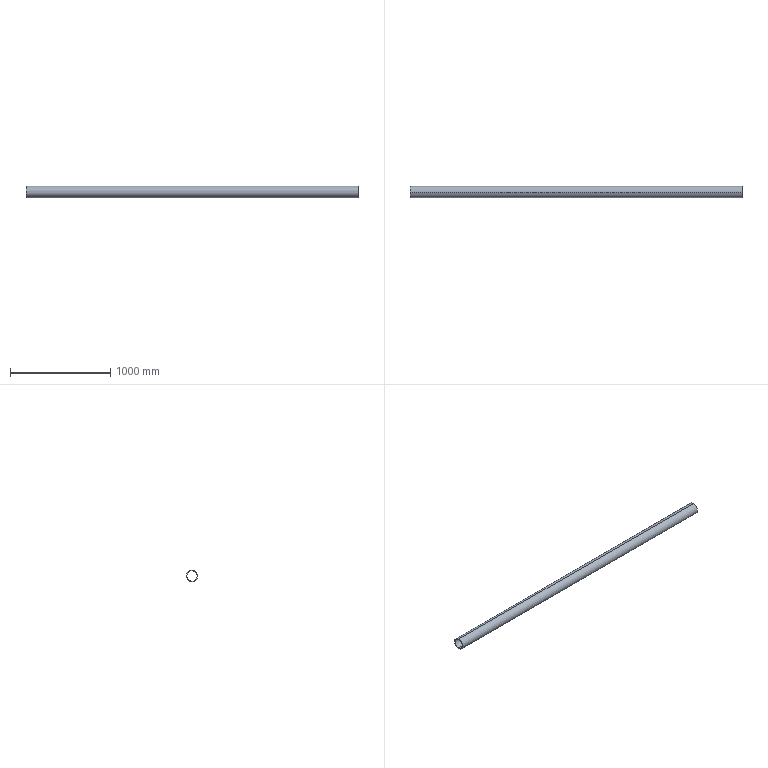Part | STEP file | Input 121 | 1 solid | 6 faces | box 3309 x 114.3 x 114.3 mm | volume 6776281 mm3 | cylinder 4 | plane 2 | commonest cylinder face diameters 102.26 x2 114.3 x2
STEP:
#1=CARTESIAN_POINT('',(0.,0.,0.));
#2=DIRECTION('',(0.,0.,1.));
#3=DIRECTION('',(1.,0.,0.));
#4=AXIS2_PLACEMENT_3D('',#1,#2,#3);
#5=CARTESIAN_POINT('',(3812.,-1.204,51.116));
#6=VERTEX_POINT('',#5);
#7=CARTESIAN_POINT('',(503.,-1.204,51.116));
#8=VERTEX_POINT('',#7);
#9=CARTESIAN_POINT('',(3812.,-1.204,51.116));
#10=DIRECTION('',(-1.,0.,0.));
#11=VECTOR('',#10,1.);
#12=LINE('',#9,#11);
#13=CARTESIAN_POINT('',(3812.,0.,0.));
#14=DIRECTION('',(-1.,0.,0.));
#15=DIRECTION('',(0.,-0.02354,0.9997));
#16=AXIS2_PLACEMENT_3D('',#13,#14,#15);
#17=CYLINDRICAL_SURFACE('',#16,51.13);
#18=CARTESIAN_POINT('',(6.283,0.));
#19=DIRECTION('',(0.,1.));
#20=VECTOR('',#19,1.);
#21=LINE('',#18,#20);
#22=(GEOMETRIC_REPRESENTATION_CONTEXT(2)PARAMETRIC_REPRESENTATION_CONTEXT()REPRESENTATION_CONTEXT('',''));
#23=DEFINITIONAL_REPRESENTATION('',(#21),#22);
#24=PCURVE('',#17,#23);
#25=CARTESIAN_POINT('',(3812.,0.,0.));
#26=DIRECTION('',(-1.,0.,0.));
#27=DIRECTION('',(0.,-0.02354,0.9997));
#28=AXIS2_PLACEMENT_3D('',#25,#26,#27);
#29=CYLINDRICAL_SURFACE('',#28,51.13);
#30=CARTESIAN_POINT('',(0.,0.));
#31=DIRECTION('',(0.,1.));
#32=VECTOR('',#31,1.);
#33=LINE('',#30,#32);
#34=(GEOMETRIC_REPRESENTATION_CONTEXT(2)PARAMETRIC_REPRESENTATION_CONTEXT()REPRESENTATION_CONTEXT('',''));
#35=DEFINITIONAL_REPRESENTATION('',(#33),#34);
#36=PCURVE('',#29,#35);
#37=SURFACE_CURVE('',#12,(#24,#36),.PCURVE_S1.);
#38=EDGE_CURVE('',#6,#8,#37,.T.);
#39=ORIENTED_EDGE('',*,*,#38,.T.);
#40=CARTESIAN_POINT('',(503.,1.204,-51.116));
#41=VERTEX_POINT('',#40);
#42=CARTESIAN_POINT('',(503.,0.,0.));
#43=DIRECTION('',(-1.,0.,0.));
#44=DIRECTION('',(0.,-0.02354,0.9997));
#45=AXIS2_PLACEMENT_3D('',#42,#43,#44);
#46=CIRCLE('',#45,51.13);
#47=CARTESIAN_POINT('',(0.,3309.));
#48=DIRECTION('',(1.,0.));
#49=VECTOR('',#48,1.);
#50=LINE('',#47,#49);
#51=(GEOMETRIC_REPRESENTATION_CONTEXT(2)PARAMETRIC_REPRESENTATION_CONTEXT()REPRESENTATION_CONTEXT('',''));
#52=DEFINITIONAL_REPRESENTATION('',(#50),#51);
#53=PCURVE('',#17,#52);
#54=CARTESIAN_POINT('',(503.,0.,0.));
#55=DIRECTION('',(-1.,0.,0.));
#56=DIRECTION('',(0.,-0.02354,0.9997));
#57=AXIS2_PLACEMENT_3D('',#54,#55,#56);
#58=PLANE('',#57);
#59=CARTESIAN_POINT('',(0.,0.));
#60=DIRECTION('',(1.,0.));
#61=AXIS2_PLACEMENT_2D('',#59,#60);
#62=CIRCLE('',#61,51.13);
#63=(GEOMETRIC_REPRESENTATION_CONTEXT(2)PARAMETRIC_REPRESENTATION_CONTEXT()REPRESENTATION_CONTEXT('',''));
#64=DEFINITIONAL_REPRESENTATION('',(#62),#63);
#65=PCURVE('',#58,#64);
#66=SURFACE_CURVE('',#46,(#53,#65),.PCURVE_S1.);
#67=EDGE_CURVE('',#41,#8,#66,.T.);
#68=ORIENTED_EDGE('',*,*,#67,.F.);
#69=CARTESIAN_POINT('',(3812.,1.204,-51.116));
#70=VERTEX_POINT('',#69);
#71=CARTESIAN_POINT('',(3812.,1.204,-51.116));
#72=DIRECTION('',(-1.,0.,0.));
#73=VECTOR('',#72,1.);
#74=LINE('',#71,#73);
#75=CARTESIAN_POINT('',(3.142,0.));
#76=DIRECTION('',(0.,1.));
#77=VECTOR('',#76,1.);
#78=LINE('',#75,#77);
#79=(GEOMETRIC_REPRESENTATION_CONTEXT(2)PARAMETRIC_REPRESENTATION_CONTEXT()REPRESENTATION_CONTEXT('',''));
#80=DEFINITIONAL_REPRESENTATION('',(#78),#79);
#81=PCURVE('',#17,#80);
#82=CARTESIAN_POINT('',(3.142,0.));
#83=DIRECTION('',(0.,1.));
#84=VECTOR('',#83,1.);
#85=LINE('',#82,#84);
#86=(GEOMETRIC_REPRESENTATION_CONTEXT(2)PARAMETRIC_REPRESENTATION_CONTEXT()REPRESENTATION_CONTEXT('',''));
#87=DEFINITIONAL_REPRESENTATION('',(#85),#86);
#88=PCURVE('',#29,#87);
#89=SURFACE_CURVE('',#74,(#81,#88),.PCURVE_S1.);
#90=EDGE_CURVE('',#70,#41,#89,.T.);
#91=ORIENTED_EDGE('',*,*,#90,.F.);
#92=CARTESIAN_POINT('',(3812.,0.,0.));
#93=DIRECTION('',(-1.,0.,0.));
#94=DIRECTION('',(0.,-0.02354,0.9997));
#95=AXIS2_PLACEMENT_3D('',#92,#93,#94);
#96=CIRCLE('',#95,51.13);
#97=CARTESIAN_POINT('',(0.,0.));
#98=DIRECTION('',(1.,0.));
#99=VECTOR('',#98,1.);
#100=LINE('',#97,#99);
#101=(GEOMETRIC_REPRESENTATION_CONTEXT(2)PARAMETRIC_REPRESENTATION_CONTEXT()REPRESENTATION_CONTEXT('',''));
#102=DEFINITIONAL_REPRESENTATION('',(#100),#101);
#103=PCURVE('',#17,#102);
#104=CARTESIAN_POINT('',(3812.,0.,0.));
#105=DIRECTION('',(-1.,0.,0.));
#106=DIRECTION('',(0.,-0.02354,0.9997));
#107=AXIS2_PLACEMENT_3D('',#104,#105,#106);
#108=PLANE('',#107);
#109=CARTESIAN_POINT('',(0.,0.));
#110=DIRECTION('',(1.,0.));
#111=AXIS2_PLACEMENT_2D('',#109,#110);
#112=CIRCLE('',#111,51.13);
#113=(GEOMETRIC_REPRESENTATION_CONTEXT(2)PARAMETRIC_REPRESENTATION_CONTEXT()REPRESENTATION_CONTEXT('',''));
#114=DEFINITIONAL_REPRESENTATION('',(#112),#113);
#115=PCURVE('',#108,#114);
#116=SURFACE_CURVE('',#96,(#103,#115),.PCURVE_S1.);
#117=EDGE_CURVE('',#70,#6,#116,.T.);
#118=ORIENTED_EDGE('',*,*,#117,.T.);
#119=EDGE_LOOP('',(#39,#68,#91,#118));
#120=FACE_BOUND('',#119,.F.);
#121=ADVANCED_FACE('',(#120),#17,.F.);
#122=CARTESIAN_POINT('',(3812.,-1.346,57.134));
#123=VERTEX_POINT('',#122);
#124=CARTESIAN_POINT('',(3812.,1.346,-57.134));
#125=VERTEX_POINT('',#124);
#126=CARTESIAN_POINT('',(3812.,0.,0.));
#127=DIRECTION('',(-1.,0.,0.));
#128=DIRECTION('',(0.,-0.02354,0.9997));
#129=AXIS2_PLACEMENT_3D('',#126,#127,#128);
#130=CIRCLE('',#129,57.15);
#131=CARTESIAN_POINT('',(3812.,0.,0.));
#132=DIRECTION('',(-1.,0.,0.));
#133=DIRECTION('',(0.,-0.02354,0.9997));
#134=AXIS2_PLACEMENT_3D('',#131,#132,#133);
#135=CYLINDRICAL_SURFACE('',#134,57.15);
#136=CARTESIAN_POINT('',(0.,0.));
#137=DIRECTION('',(1.,0.));
#138=VECTOR('',#137,1.);
#139=LINE('',#136,#138);
#140=(GEOMETRIC_REPRESENTATION_CONTEXT(2)PARAMETRIC_REPRESENTATION_CONTEXT()REPRESENTATION_CONTEXT('',''));
#141=DEFINITIONAL_REPRESENTATION('',(#139),#140);
#142=PCURVE('',#135,#141);
#143=CARTESIAN_POINT('',(0.,0.));
#144=DIRECTION('',(1.,0.));
#145=AXIS2_PLACEMENT_2D('',#143,#144);
#146=CIRCLE('',#145,57.15);
#147=(GEOMETRIC_REPRESENTATION_CONTEXT(2)PARAMETRIC_REPRESENTATION_CONTEXT()REPRESENTATION_CONTEXT('',''));
#148=DEFINITIONAL_REPRESENTATION('',(#146),#147);
#149=PCURVE('',#108,#148);
#150=SURFACE_CURVE('',#130,(#142,#149),.PCURVE_S1.);
#151=EDGE_CURVE('',#123,#125,#150,.T.);
#152=ORIENTED_EDGE('',*,*,#151,.T.);
#153=CARTESIAN_POINT('',(503.,1.346,-57.134));
#154=VERTEX_POINT('',#153);
#155=CARTESIAN_POINT('',(3812.,1.346,-57.134));
#156=DIRECTION('',(-1.,0.,0.));
#157=VECTOR('',#156,1.);
#158=LINE('',#155,#157);
#159=CARTESIAN_POINT('',(3.142,0.));
#160=DIRECTION('',(0.,1.));
#161=VECTOR('',#160,1.);
#162=LINE('',#159,#161);
#163=(GEOMETRIC_REPRESENTATION_CONTEXT(2)PARAMETRIC_REPRESENTATION_CONTEXT()REPRESENTATION_CONTEXT('',''));
#164=DEFINITIONAL_REPRESENTATION('',(#162),#163);
#165=PCURVE('',#135,#164);
#166=CARTESIAN_POINT('',(3812.,0.,0.));
#167=DIRECTION('',(-1.,0.,0.));
#168=DIRECTION('',(0.,-0.02354,0.9997));
#169=AXIS2_PLACEMENT_3D('',#166,#167,#168);
#170=CYLINDRICAL_SURFACE('',#169,57.15);
#171=CARTESIAN_POINT('',(3.142,0.));
#172=DIRECTION('',(0.,1.));
#173=VECTOR('',#172,1.);
#174=LINE('',#171,#173);
#175=(GEOMETRIC_REPRESENTATION_CONTEXT(2)PARAMETRIC_REPRESENTATION_CONTEXT()REPRESENTATION_CONTEXT('',''));
#176=DEFINITIONAL_REPRESENTATION('',(#174),#175);
#177=PCURVE('',#170,#176);
#178=SURFACE_CURVE('',#158,(#165,#177),.PCURVE_S1.);
#179=EDGE_CURVE('',#125,#154,#178,.T.);
#180=ORIENTED_EDGE('',*,*,#179,.T.);
#181=CARTESIAN_POINT('',(503.,-1.346,57.134));
#182=VERTEX_POINT('',#181);
#183=CARTESIAN_POINT('',(503.,0.,0.));
#184=DIRECTION('',(-1.,0.,0.));
#185=DIRECTION('',(0.,-0.02354,0.9997));
#186=AXIS2_PLACEMENT_3D('',#183,#184,#185);
#187=CIRCLE('',#186,57.15);
#188=CARTESIAN_POINT('',(0.,3309.));
#189=DIRECTION('',(1.,0.));
#190=VECTOR('',#189,1.);
#191=LINE('',#188,#190);
#192=(GEOMETRIC_REPRESENTATION_CONTEXT(2)PARAMETRIC_REPRESENTATION_CONTEXT()REPRESENTATION_CONTEXT('',''));
#193=DEFINITIONAL_REPRESENTATION('',(#191),#192);
#194=PCURVE('',#135,#193);
#195=CARTESIAN_POINT('',(0.,0.));
#196=DIRECTION('',(1.,0.));
#197=AXIS2_PLACEMENT_2D('',#195,#196);
#198=CIRCLE('',#197,57.15);
#199=(GEOMETRIC_REPRESENTATION_CONTEXT(2)PARAMETRIC_REPRESENTATION_CONTEXT()REPRESENTATION_CONTEXT('',''));
#200=DEFINITIONAL_REPRESENTATION('',(#198),#199);
#201=PCURVE('',#58,#200);
#202=SURFACE_CURVE('',#187,(#194,#201),.PCURVE_S1.);
#203=EDGE_CURVE('',#182,#154,#202,.T.);
#204=ORIENTED_EDGE('',*,*,#203,.F.);
#205=CARTESIAN_POINT('',(3812.,-1.346,57.134));
#206=DIRECTION('',(-1.,0.,0.));
#207=VECTOR('',#206,1.);
#208=LINE('',#205,#207);
#209=CARTESIAN_POINT('',(0.,0.));
#210=DIRECTION('',(0.,1.));
#211=VECTOR('',#210,1.);
#212=LINE('',#209,#211);
#213=(GEOMETRIC_REPRESENTATION_CONTEXT(2)PARAMETRIC_REPRESENTATION_CONTEXT()REPRESENTATION_CONTEXT('',''));
#214=DEFINITIONAL_REPRESENTATION('',(#212),#213);
#215=PCURVE('',#135,#214);
#216=CARTESIAN_POINT('',(6.283,0.));
#217=DIRECTION('',(0.,1.));
#218=VECTOR('',#217,1.);
#219=LINE('',#216,#218);
#220=(GEOMETRIC_REPRESENTATION_CONTEXT(2)PARAMETRIC_REPRESENTATION_CONTEXT()REPRESENTATION_CONTEXT('',''));
#221=DEFINITIONAL_REPRESENTATION('',(#219),#220);
#222=PCURVE('',#170,#221);
#223=SURFACE_CURVE('',#208,(#215,#222),.PCURVE_S1.);
#224=EDGE_CURVE('',#123,#182,#223,.T.);
#225=ORIENTED_EDGE('',*,*,#224,.F.);
#226=EDGE_LOOP('',(#152,#180,#204,#225));
#227=FACE_BOUND('',#226,.T.);
#228=ADVANCED_FACE('',(#227),#135,.T.);
#229=ORIENTED_EDGE('',*,*,#179,.F.);
#230=CARTESIAN_POINT('',(3812.,0.,0.));
#231=DIRECTION('',(-1.,0.,0.));
#232=DIRECTION('',(0.,-0.02354,0.9997));
#233=AXIS2_PLACEMENT_3D('',#230,#231,#232);
#234=CIRCLE('',#233,57.15);
#235=CARTESIAN_POINT('',(0.,0.));
#236=DIRECTION('',(1.,0.));
#237=VECTOR('',#236,1.);
#238=LINE('',#235,#237);
#239=(GEOMETRIC_REPRESENTATION_CONTEXT(2)PARAMETRIC_REPRESENTATION_CONTEXT()REPRESENTATION_CONTEXT('',''));
#240=DEFINITIONAL_REPRESENTATION('',(#238),#239);
#241=PCURVE('',#170,#240);
#242=CARTESIAN_POINT('',(0.,0.));
#243=DIRECTION('',(1.,0.));
#244=AXIS2_PLACEMENT_2D('',#242,#243);
#245=CIRCLE('',#244,57.15);
#246=(GEOMETRIC_REPRESENTATION_CONTEXT(2)PARAMETRIC_REPRESENTATION_CONTEXT()REPRESENTATION_CONTEXT('',''));
#247=DEFINITIONAL_REPRESENTATION('',(#245),#246);
#248=PCURVE('',#108,#247);
#249=SURFACE_CURVE('',#234,(#241,#248),.PCURVE_S1.);
#250=EDGE_CURVE('',#125,#123,#249,.T.);
#251=ORIENTED_EDGE('',*,*,#250,.T.);
#252=ORIENTED_EDGE('',*,*,#224,.T.);
#253=CARTESIAN_POINT('',(503.,0.,0.));
#254=DIRECTION('',(-1.,0.,0.));
#255=DIRECTION('',(0.,-0.02354,0.9997));
#256=AXIS2_PLACEMENT_3D('',#253,#254,#255);
#257=CIRCLE('',#256,57.15);
#258=CARTESIAN_POINT('',(0.,3309.));
#259=DIRECTION('',(1.,0.));
#260=VECTOR('',#259,1.);
#261=LINE('',#258,#260);
#262=(GEOMETRIC_REPRESENTATION_CONTEXT(2)PARAMETRIC_REPRESENTATION_CONTEXT()REPRESENTATION_CONTEXT('',''));
#263=DEFINITIONAL_REPRESENTATION('',(#261),#262);
#264=PCURVE('',#170,#263);
#265=CARTESIAN_POINT('',(0.,0.));
#266=DIRECTION('',(1.,0.));
#267=AXIS2_PLACEMENT_2D('',#265,#266);
#268=CIRCLE('',#267,57.15);
#269=(GEOMETRIC_REPRESENTATION_CONTEXT(2)PARAMETRIC_REPRESENTATION_CONTEXT()REPRESENTATION_CONTEXT('',''));
#270=DEFINITIONAL_REPRESENTATION('',(#268),#269);
#271=PCURVE('',#58,#270);
#272=SURFACE_CURVE('',#257,(#264,#271),.PCURVE_S1.);
#273=EDGE_CURVE('',#154,#182,#272,.T.);
#274=ORIENTED_EDGE('',*,*,#273,.F.);
#275=EDGE_LOOP('',(#229,#251,#252,#274));
#276=FACE_BOUND('',#275,.T.);
#277=ADVANCED_FACE('',(#276),#170,.T.);
#278=CARTESIAN_POINT('',(3812.,0.,0.));
#279=DIRECTION('',(-1.,0.,0.));
#280=DIRECTION('',(0.,-0.02354,0.9997));
#281=AXIS2_PLACEMENT_3D('',#278,#279,#280);
#282=CIRCLE('',#281,51.13);
#283=CARTESIAN_POINT('',(0.,0.));
#284=DIRECTION('',(1.,0.));
#285=AXIS2_PLACEMENT_2D('',#283,#284);
#286=CIRCLE('',#285,51.13);
#287=(GEOMETRIC_REPRESENTATION_CONTEXT(2)PARAMETRIC_REPRESENTATION_CONTEXT()REPRESENTATION_CONTEXT('',''));
#288=DEFINITIONAL_REPRESENTATION('',(#286),#287);
#289=PCURVE('',#108,#288);
#290=CARTESIAN_POINT('',(0.,0.));
#291=DIRECTION('',(1.,0.));
#292=VECTOR('',#291,1.);
#293=LINE('',#290,#292);
#294=(GEOMETRIC_REPRESENTATION_CONTEXT(2)PARAMETRIC_REPRESENTATION_CONTEXT()REPRESENTATION_CONTEXT('',''));
#295=DEFINITIONAL_REPRESENTATION('',(#293),#294);
#296=PCURVE('',#29,#295);
#297=SURFACE_CURVE('',#282,(#289,#296),.PCURVE_S1.);
#298=EDGE_CURVE('',#6,#70,#297,.T.);
#299=ORIENTED_EDGE('',*,*,#298,.T.);
#300=ORIENTED_EDGE('',*,*,#117,.T.);
#301=EDGE_LOOP('',(#299,#300));
#302=FACE_BOUND('',#301,.T.);
#303=ORIENTED_EDGE('',*,*,#151,.F.);
#304=ORIENTED_EDGE('',*,*,#250,.F.);
#305=EDGE_LOOP('',(#303,#304));
#306=FACE_BOUND('',#305,.T.);
#307=ADVANCED_FACE('',(#302,#306),#108,.F.);
#308=CARTESIAN_POINT('',(503.,0.,0.));
#309=DIRECTION('',(-1.,0.,0.));
#310=DIRECTION('',(0.,-0.02354,0.9997));
#311=AXIS2_PLACEMENT_3D('',#308,#309,#310);
#312=CIRCLE('',#311,51.13);
#313=CARTESIAN_POINT('',(0.,0.));
#314=DIRECTION('',(1.,0.));
#315=AXIS2_PLACEMENT_2D('',#313,#314);
#316=CIRCLE('',#315,51.13);
#317=(GEOMETRIC_REPRESENTATION_CONTEXT(2)PARAMETRIC_REPRESENTATION_CONTEXT()REPRESENTATION_CONTEXT('',''));
#318=DEFINITIONAL_REPRESENTATION('',(#316),#317);
#319=PCURVE('',#58,#318);
#320=CARTESIAN_POINT('',(0.,3309.));
#321=DIRECTION('',(1.,0.));
#322=VECTOR('',#321,1.);
#323=LINE('',#320,#322);
#324=(GEOMETRIC_REPRESENTATION_CONTEXT(2)PARAMETRIC_REPRESENTATION_CONTEXT()REPRESENTATION_CONTEXT('',''));
#325=DEFINITIONAL_REPRESENTATION('',(#323),#324);
#326=PCURVE('',#29,#325);
#327=SURFACE_CURVE('',#312,(#319,#326),.PCURVE_S1.);
#328=EDGE_CURVE('',#8,#41,#327,.T.);
#329=ORIENTED_EDGE('',*,*,#328,.F.);
#330=ORIENTED_EDGE('',*,*,#67,.F.);
#331=EDGE_LOOP('',(#329,#330));
#332=FACE_BOUND('',#331,.T.);
#333=ORIENTED_EDGE('',*,*,#203,.T.);
#334=ORIENTED_EDGE('',*,*,#273,.T.);
#335=EDGE_LOOP('',(#333,#334));
#336=FACE_BOUND('',#335,.T.);
#337=ADVANCED_FACE('',(#332,#336),#58,.T.);
#338=ORIENTED_EDGE('',*,*,#328,.F.);
#339=ORIENTED_EDGE('',*,*,#38,.F.);
#340=ORIENTED_EDGE('',*,*,#298,.T.);
#341=ORIENTED_EDGE('',*,*,#90,.T.);
#342=EDGE_LOOP('',(#338,#339,#340,#341));
#343=FACE_BOUND('',#342,.F.);
#344=ADVANCED_FACE('',(#343),#29,.F.);
#345=CLOSED_SHELL('',(#121,#228,#277,#307,#337,#344));
#346=MANIFOLD_SOLID_BREP('',#345);
#347=(LENGTH_UNIT()NAMED_UNIT(*)SI_UNIT(.MILLI.,.METRE.));
#348=UNCERTAINTY_MEASURE_WITH_UNIT(LENGTH_MEASURE(0.0000001),#347,'','');
#349=(NAMED_UNIT(*)PLANE_ANGLE_UNIT()SI_UNIT($,.RADIAN.));
#350=(NAMED_UNIT(*)SI_UNIT($,.STERADIAN.)SOLID_ANGLE_UNIT());
#351=(GEOMETRIC_REPRESENTATION_CONTEXT(3)GLOBAL_UNCERTAINTY_ASSIGNED_CONTEXT((#348))GLOBAL_UNIT_ASSIGNED_CONTEXT((#347,#349,#350))REPRESENTATION_CONTEXT('',''));
#352=ADVANCED_BREP_SHAPE_REPRESENTATION('',(#4,#346),#351);